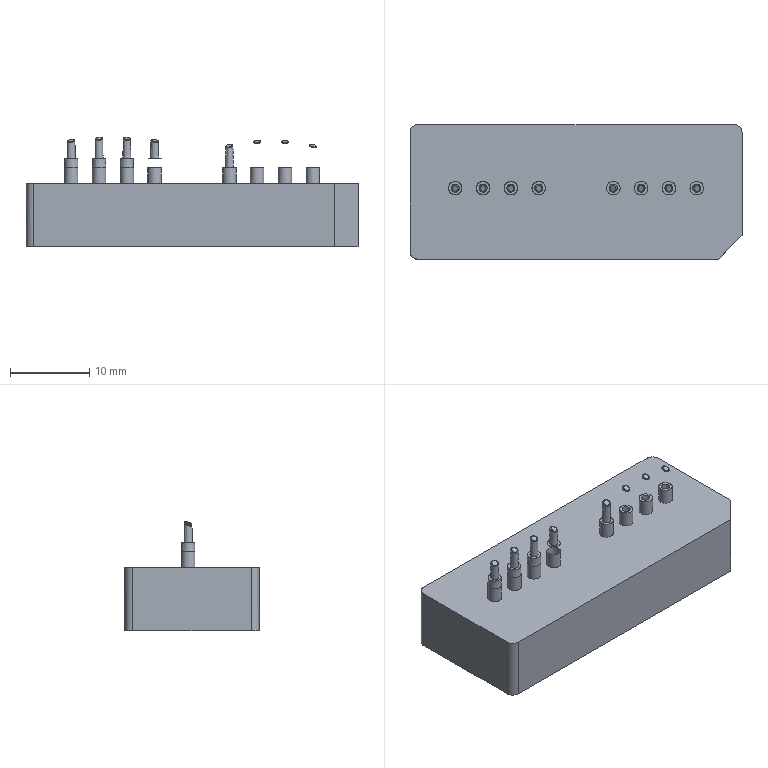NC program | PowerMill | posted by the shop | part box 42 x 17 x 13.856 mm
Lines 29045 to 29939 of 273708:
( TOOL ID   D10_1_1 )
( TOOL DIA. 10. TIP RAD 0 LENGTH 69. )
( Z = -6.06 )
T3 M6
T6
G91 G28 Z0
G0 G90 G54
M08
S8500 M3
X0 Y0 M8
G43 Z9.79 H3
X20.336 Y19.268
Z-4.86
G1 Z-6.06 F360
X20.127 Y13.997 F600
X6.597
X.484 Y5.107
X.565 Y5.157
X.642 Y5.215
X.852 Y5.391
X1.136 Y5.602
X1.42 Y5.789
X1.709 Y5.959
X1.987 Y6.103
X2.273 Y6.233
X2.555 Y6.346
X2.839 Y6.443
X3.128 Y6.526
X3.409 Y6.594
X3.691 Y6.647
X3.975 Y6.688
X4.259 Y6.716
X4.543 Y6.731
X4.826 Y6.732
X5.11 Y6.721
X5.394 Y6.697
X5.678 Y6.66
X5.962 Y6.61
X6.257 Y6.541
G3 X6.703 Y6.539 I.227 J.974
G1 X7.098 Y6.628
X7.382 Y6.674
X7.666 Y6.707
X7.95 Y6.726
X8.233 Y6.733
X8.517 Y6.727
X8.801 Y6.708
X9.085 Y6.676
X9.369 Y6.631
X9.598 Y6.584
X9.764 Y6.544
G3 X10.229 Y6.542 I.237 J.971
G1 X10.505 Y6.606
X10.789 Y6.658
X11.073 Y6.696
X11.356 Y6.72
X11.64 Y6.732
X11.924 Y6.731
X12.208 Y6.717
X12.492 Y6.69
X12.776 Y6.65
X13.06 Y6.596
X13.287 Y6.543
G3 X13.755 Y6.544 I.23 J.973
G1 X13.912 Y6.583
X14.196 Y6.639
X14.479 Y6.683
X14.763 Y6.712
X15.047 Y6.729
X15.331 Y6.733
X15.615 Y6.724
X15.899 Y6.702
X16.183 Y6.667
X16.467 Y6.619
X16.751 Y6.557
X17.095 Y6.463
X17.319 Y6.39
X17.601 Y6.286
X17.886 Y6.163
X18.086 Y6.067
X18.291 Y5.959
X18.454 Y5.866
X18.737 Y5.689
X19.022 Y5.488
X19.148 Y5.391
X19.355 Y5.221
X19.59 Y5.008
X19.796 Y4.802
X19.988 Y4.592
X20.158 Y4.39
X20.262 Y4.256
X20.466 Y3.971
X20.645 Y3.689
X20.726 Y3.55
X20.843 Y3.332
X20.946 Y3.121
X21.071 Y2.836
X21.177 Y2.554
G2 X21.347 Y1.986 I-5.759 J-2.034
G1 X21.411 Y1.703
X21.461 Y1.419
X21.497 Y1.135
X21.521 Y.851
X21.532 Y.568
X21.529 Y.284
X21.514 Y0
X21.486 Y-.284
X21.444 Y-.568
X21.389 Y-.851
X21.293 Y-1.234
X21.238 Y-1.419
X21.14 Y-1.703
X21.027 Y-1.986
X20.897 Y-2.27
X20.726 Y-2.595
X20.568 Y-2.858
X20.393 Y-3.121
X20.158 Y-3.435
X19.952 Y-3.679
X19.774 Y-3.871
X19.571 Y-4.071
X19.366 Y-4.256
X19.022 Y-4.533
X18.806 Y-4.688
X18.607 Y-4.818
X18.404 Y-4.939
X18.17 Y-5.069
X17.886 Y-5.208
X17.663 Y-5.305
X17.443 Y-5.391
X17.319 Y-5.436
X17.035 Y-5.526
X16.751 Y-5.602
X16.467 Y-5.664
X16.183 Y-5.712
X15.899 Y-5.747
X15.615 Y-5.769
X15.331 Y-5.778
X15.047 Y-5.774
X14.763 Y-5.758
X14.479 Y-5.727
X14.196 Y-5.684
X13.912 Y-5.628
X13.759 Y-5.59
G3 X13.288 Y-5.587 I-.241 J-.971
G1 X13.06 Y-5.641
X12.776 Y-5.695
X12.492 Y-5.735
X12.208 Y-5.762
X11.924 Y-5.776
X11.64 Y-5.777
X11.362 Y-5.766
X11.073 Y-5.741
X10.789 Y-5.703
X10.505 Y-5.651
X10.221 Y-5.586
G3 X9.749 Y-5.592 I-.224 J-.975
G1 X9.653 Y-5.617
X9.369 Y-5.676
X9.085 Y-5.721
X8.801 Y-5.753
X8.517 Y-5.772
X8.233 Y-5.778
X7.95 Y-5.772
X7.666 Y-5.752
X7.382 Y-5.719
X7.098 Y-5.673
X6.814 Y-5.613
X6.736 Y-5.593
G3 X6.246 Y-5.59 I-.251 J-.968
G1 X5.962 Y-5.654
X5.678 Y-5.705
X5.394 Y-5.742
X5.11 Y-5.766
X4.826 Y-5.778
X4.543 Y-5.776
X4.259 Y-5.761
X3.975 Y-5.734
X3.691 Y-5.692
X3.407 Y-5.638
X3.123 Y-5.57
X2.84 Y-5.488
X2.555 Y-5.39
X2.271 Y-5.278
X1.987 Y-5.148
X1.703 Y-5.001
X1.42 Y-4.835
X1.127 Y-4.641
X.852 Y-4.436
X.636 Y-4.258
G3 X-.636 Y-4.258 I-.636 J-.771
G1 X-.852 Y-4.436
X-1.127 Y-4.641
X-1.42 Y-4.835
X-1.703 Y-5.001
X-1.987 Y-5.148
X-2.271 Y-5.278
X-2.555 Y-5.39
X-2.84 Y-5.488
X-3.123 Y-5.57
X-3.407 Y-5.638
X-3.691 Y-5.692
X-3.975 Y-5.733
X-4.259 Y-5.761
X-4.543 Y-5.776
X-4.826 Y-5.778
X-5.11 Y-5.766
X-5.394 Y-5.742
X-5.678 Y-5.705
X-5.962 Y-5.654
X-6.246 Y-5.59
G3 X-6.736 Y-5.593 I-.239 J-.971
G1 X-6.814 Y-5.613
X-7.098 Y-5.673
X-7.382 Y-5.719
X-7.666 Y-5.752
X-7.95 Y-5.771
X-8.233 Y-5.778
X-8.517 Y-5.772
X-8.801 Y-5.753
X-9.085 Y-5.721
X-9.369 Y-5.676
X-9.653 Y-5.617
X-9.749 Y-5.592
G3 X-10.221 Y-5.586 I-.248 J-.969
G1 X-10.505 Y-5.651
X-10.789 Y-5.703
X-11.073 Y-5.741
X-11.363 Y-5.766
X-11.64 Y-5.777
X-11.924 Y-5.776
X-12.208 Y-5.762
X-12.492 Y-5.735
X-12.776 Y-5.695
X-13.06 Y-5.641
X-13.288 Y-5.587
G3 X-13.759 Y-5.59 I-.231 J-.973
G1 X-13.912 Y-5.628
X-14.196 Y-5.684
X-14.479 Y-5.727
X-14.763 Y-5.758
X-15.047 Y-5.774
X-15.331 Y-5.778
X-15.615 Y-5.769
X-15.899 Y-5.747
X-16.183 Y-5.712
X-16.467 Y-5.664
X-16.751 Y-5.602
X-17.035 Y-5.526
X-17.319 Y-5.436
X-17.661 Y-5.306
X-17.886 Y-5.208
X-18.17 Y-5.069
X-18.454 Y-4.911
X-18.598 Y-4.824
X-18.81 Y-4.685
X-19.022 Y-4.533
X-19.176 Y-4.414
X-19.366 Y-4.256
X-19.59 Y-4.053
X-19.774 Y-3.871
X-19.952 Y-3.679
X-20.158 Y-3.435
X-20.393 Y-3.121
X-20.569 Y-2.858
X-20.749 Y-2.554
X-20.896 Y-2.27
X-21.027 Y-1.986
X-21.14 Y-1.703
X-21.266 Y-1.326
X-21.293 Y-1.234
X-21.389 Y-.851
X-21.444 Y-.568
X-21.485 Y-.284
X-21.514 Y0
X-21.529 Y.284
X-21.531 Y.568
X-21.521 Y.851
X-21.498 Y1.135
X-21.461 Y1.419
X-21.411 Y1.703
X-21.347 Y1.986
G2 X-21.177 Y2.554 I6.096 J-1.516
G1 X-21.07 Y2.838
X-20.946 Y3.121
X-20.841 Y3.336
X-20.726 Y3.55
X-20.645 Y3.689
X-20.465 Y3.973
X-20.262 Y4.256
X-20.158 Y4.39
X-20.008 Y4.57
X-19.776 Y4.824
X-19.59 Y5.008
X-19.359 Y5.217
X-19.148 Y5.391
X-19.022 Y5.488
X-18.728 Y5.695
X-18.454 Y5.866
X-18.291 Y5.959
X-17.886 Y6.163
X-17.588 Y6.29
X-17.319 Y6.39
X-17.095 Y6.463
X-16.872 Y6.526
X-16.467 Y6.619
X-16.183 Y6.667
X-15.899 Y6.702
X-15.615 Y6.724
X-15.331 Y6.733
X-15.047 Y6.729
X-14.763 Y6.712
X-14.479 Y6.682
X-14.196 Y6.639
X-13.912 Y6.583
X-13.75 Y6.544
G3 X-13.286 Y6.543 I.234 J.972
G1 X-13.06 Y6.596
X-12.776 Y6.65
X-12.492 Y6.69
X-12.208 Y6.717
X-11.924 Y6.731
X-11.64 Y6.732
X-11.356 Y6.72
X-11.073 Y6.696
X-10.789 Y6.658
X-10.505 Y6.606
X-10.227 Y6.541
G3 X-9.781 Y6.539 I.228 J.974
G1 X-9.369 Y6.631
X-9.085 Y6.676
X-8.801 Y6.708
X-8.517 Y6.727
X-8.233 Y6.733
X-7.95 Y6.726
X-7.666 Y6.707
X-7.382 Y6.674
X-7.098 Y6.628
X-6.703 Y6.539
G3 X-6.256 Y6.541 I.219 J.976
G1 X-5.962 Y6.61
X-5.678 Y6.66
X-5.394 Y6.697
X-5.11 Y6.721
X-4.826 Y6.732
X-4.543 Y6.731
X-4.259 Y6.716
X-3.975 Y6.688
X-3.691 Y6.647
X-3.409 Y6.594
X-3.123 Y6.525
X-2.839 Y6.443
X-2.555 Y6.345
X-2.285 Y6.239
X-1.987 Y6.103
X-1.709 Y5.959
X-1.42 Y5.789
X-1.155 Y5.615
X-.852 Y5.391
X-.64 Y5.214
G3 X.484 Y5.107 I.641 J.768
G0 Z9.79
X0 Y0
X25.987 Y-14.768
Z-12.76
G1 Z-13.96 F360
G3 X22.452 Y-11.232 I-1.768 J1.768 F600
G1 X21.614 Y-12.07
X21.613 Y-12.071
X21.395 Y-12.279
X21.394 Y-12.28
X21.392 Y-12.281
X21.267 Y-12.39
X21.266 Y-12.391
X21.265 Y-12.392
X21.074 Y-12.545
X21.072 Y-12.546
X21.07 Y-12.547
X20.842 Y-12.711
X20.84 Y-12.712
X20.839 Y-12.713
X20.752 Y-12.77
X20.75 Y-12.771
X20.748 Y-12.772
X20.432 Y-12.96
X20.43 Y-12.961
X20.429 Y-12.962
X20.293 Y-13.033
X20.292
X20.291 Y-13.034
X20.11 Y-13.121
X20.108 Y-13.122
X20.106 Y-13.123
X19.79 Y-13.254
X19.787 Y-13.255
X19.785 Y-13.256
X19.499 Y-13.354
X19.496 Y-13.355
X19.494
X19.148 Y-13.449
X19.145
X19.142 Y-13.45
X18.826 Y-13.512
X18.824 Y-13.513
X18.821
X18.505 Y-13.555
X18.502
X18.5
X18.184 Y-13.577
X18.181
X18.179
X17.863 Y-13.58
X17.862
X-20.075 Y-13.579
X-20.077
X-20.078
X-20.394 Y-13.567
X-20.397
X-20.399
X-20.715 Y-13.538
X-20.717 Y-13.537
X-20.719
X-21.035 Y-13.491
X-21.037
X-21.039 Y-13.49
X-21.356 Y-13.427
X-21.358 Y-13.426
X-21.36
X-21.636 Y-13.356
X-21.638 Y-13.355
X-21.64 Y-13.354
X-21.996 Y-13.243
X-21.998 Y-13.242
X-22.001 Y-13.241
X-22.317 Y-13.121
X-22.319 Y-13.12
X-22.321
X-22.637 Y-12.978
X-22.639 Y-12.977
X-22.641 Y-12.976
X-22.957 Y-12.812
X-22.959 Y-12.811
X-22.961 Y-12.81
X-23.125 Y-12.715
X-23.127 Y-12.714
X-23.128
X-23.279 Y-12.62
X-23.28 Y-12.619
X-23.282 Y-12.618
X-23.598 Y-12.401
X-23.6 Y-12.399
X-23.602 Y-12.398
X-23.919 Y-12.149
X-23.92 Y-12.148
X-23.921 Y-12.147
X-24.005 Y-12.074
X-24.006 Y-12.073
X-24.008 Y-12.072
X-24.239 Y-11.858
X-24.241 Y-11.857
X-24.242 Y-11.856
X-24.344 Y-11.754
X-24.345 Y-11.753
X-24.346 Y-11.752
X-24.56 Y-11.522
X-24.561 Y-11.52
X-24.562 Y-11.519
X-24.636 Y-11.433
X-24.637 Y-11.432
Y-11.431
X-24.88 Y-11.126
X-24.882 Y-11.124
X-24.883 Y-11.122
X-25.11 Y-10.794
X-25.111 Y-10.793
X-25.112 Y-10.791
X-25.201 Y-10.648
X-25.202 Y-10.647
X-25.203 Y-10.646
X-25.303 Y-10.473
X-25.304 Y-10.471
X-25.305 Y-10.47
X-25.47 Y-10.154
X-25.471 Y-10.152
X-25.472 Y-10.149
X-25.614 Y-9.833
X-25.615 Y-9.831
X-25.616 Y-9.829
X-25.737 Y-9.513
X-25.738 Y-9.511
X-25.739 Y-9.509
X-25.84 Y-9.193
Y-9.19
X-25.841 Y-9.188
X-25.923 Y-8.872
X-25.924 Y-8.87
Y-8.868
X-25.988 Y-8.552
Y-8.55
Y-8.548
X-26.036 Y-8.232
Y-8.229
Y-8.227
X-26.065 Y-7.911
Y-7.909
X-26.066 Y-7.907
X-26.079 Y-7.591
Y-7.589
Y-7.587
Y7.587
Y7.589
Y7.591
X-26.066 Y7.907
Y7.909
Y7.911
X-26.036 Y8.227
Y8.229
Y8.231
X-25.989 Y8.548
Y8.55
X-25.988 Y8.552
X-25.924 Y8.868
Y8.87
X-25.923 Y8.872
X-25.843 Y9.179
Y9.182
X-25.842 Y9.184
X-25.738 Y9.509
Y9.511
X-25.737 Y9.513
X-25.616 Y9.829
X-25.615 Y9.831
X-25.614 Y9.833
X-25.472 Y10.149
X-25.471 Y10.152
X-25.47 Y10.154
X-25.305 Y10.47
X-25.304 Y10.471
X-25.303 Y10.473
X-25.203 Y10.646
X-25.202 Y10.647
X-25.201 Y10.648
X-25.112 Y10.791
X-25.111 Y10.793
X-25.11 Y10.794
X-24.892 Y11.111
X-24.89 Y11.113
X-24.889 Y11.115
X-24.638 Y11.431
X-24.637 Y11.432
X-24.636 Y11.434
X-24.562 Y11.519
X-24.561 Y11.521
X-24.56 Y11.522
X-24.346 Y11.752
X-24.345 Y11.753
X-24.344 Y11.754
X-24.242 Y11.856
X-24.241 Y11.857
X-24.239 Y11.858
X-24.007 Y12.072
X-24.006 Y12.073
X-24.005 Y12.074
X-23.921 Y12.146
X-23.92 Y12.147
X-23.919 Y12.148
X-23.61 Y12.392
X-23.608 Y12.394
X-23.605 Y12.396
X-23.282 Y12.618
X-23.28 Y12.619
X-23.279 Y12.62
X-23.128 Y12.714
X-23.127
X-23.125 Y12.715
X-22.961 Y12.81
X-22.959 Y12.811
X-22.957 Y12.812
X-22.641 Y12.976
X-22.639 Y12.977
X-22.637 Y12.978
X-22.321 Y13.12
X-22.319
X-22.317 Y13.121
X-22.001 Y13.241
X-21.998 Y13.242
X-21.996 Y13.243
X-21.68 Y13.343
X-21.678 Y13.344
X-21.676
X-21.36 Y13.426
X-21.358
X-21.355 Y13.427
X-21.039 Y13.49
X-21.037
X-21.035
X-20.719 Y13.537
X-20.717
X-20.715 Y13.538
X-20.399 Y13.566
X-20.397
X-20.395
X-20.079 Y13.579
X-20.077
X-20.075
X-.316
X20.075
X20.077
X20.078
X20.394 Y13.567
X20.397
X20.399
X20.715 Y13.538
X20.717 Y13.537
X20.719
X21.035 Y13.491
X21.037
X21.039 Y13.49
X21.356 Y13.427
X21.358 Y13.426
X21.36
X21.636 Y13.356
X21.638 Y13.355
X21.64 Y13.354
X21.996 Y13.243
X21.998 Y13.242
X22.001 Y13.241
X22.317 Y13.121
X22.319 Y13.12
X22.321
X22.637 Y12.978
X22.639 Y12.977
X22.641 Y12.976
X22.957 Y12.812
X22.959 Y12.811
X22.961 Y12.81
X23.125 Y12.715
X23.127 Y12.714
X23.128
X23.279 Y12.62
X23.28 Y12.619
X23.282 Y12.618
X23.598 Y12.401
X23.6 Y12.399
X23.602 Y12.398
X23.919 Y12.149
X23.92 Y12.148
X23.921 Y12.147
X24.005 Y12.074
X24.006 Y12.073
X24.008 Y12.072
X24.239 Y11.858
X24.241 Y11.857
X24.242 Y11.856
X24.344 Y11.754
X24.345 Y11.753
X24.346 Y11.752
X24.56 Y11.522
X24.561 Y11.52
X24.562 Y11.519
X24.636 Y11.433
X24.637 Y11.432
Y11.431
X24.88 Y11.126
X24.882 Y11.124
X24.883 Y11.122
X25.11 Y10.794
X25.111 Y10.793
X25.112 Y10.791
X25.201 Y10.648
X25.202 Y10.647
X25.203 Y10.646
X25.303 Y10.473
X25.304 Y10.471
X25.305 Y10.47
X25.47 Y10.154
X25.471 Y10.152
X25.472 Y10.149
X25.614 Y9.833
X25.615 Y9.831
X25.616 Y9.829
X25.737 Y9.513
X25.738 Y9.511
X25.739 Y9.509
X25.84 Y9.193
Y9.19
X25.841 Y9.188
X25.923 Y8.872
X25.924 Y8.87
Y8.868
X25.988 Y8.552
Y8.55
Y8.548
X26.036 Y8.232
Y8.229
Y8.227
X26.065 Y7.911
Y7.909
X26.066 Y7.907
X26.079 Y7.591
Y7.589
Y7.588
X26.08 Y-5.374
Y-5.375
X26.076 Y-5.692
Y-5.694
Y-5.696
X26.054 Y-6.012
Y-6.015
Y-6.017
X26.011 Y-6.334
Y-6.336
X26.01 Y-6.339
X25.947 Y-6.655
X25.946 Y-6.657
Y-6.66
X25.861 Y-6.976
X25.86 Y-6.979
X25.859 Y-6.981
X25.751 Y-7.297
Y-7.3
X25.75 Y-7.302
X25.617 Y-7.618
X25.616 Y-7.62
X25.615 Y-7.622
X25.522 Y-7.815
X25.521 Y-7.817
X25.52 Y-7.818
X25.455 Y-7.941
X25.454 Y-7.943
X25.453 Y-7.945
X25.264 Y-8.261
X25.263 Y-8.262
X25.262 Y-8.264
X25.2 Y-8.357
X25.199 Y-8.359
X25.198 Y-8.36
X25.038 Y-8.583
X25.036 Y-8.584
X25.035 Y-8.586
X24.88 Y-8.779
X24.879 Y-8.781
X24.878 Y-8.782
X24.77 Y-8.905
X24.769 Y-8.906
X24.768 Y-8.907
X24.559 Y-9.125
X24.558 Y-9.126
X22.452 Y-11.232
G3 X25.987 Y-14.768 I1.768 J-1.768
G1 X25.936 Y-14.706
G3 X22.4 Y-11.171 I-1.768 J1.768
G1 X21.558 Y-12.014
X21.34 Y-12.221
X21.215 Y-12.33
X21.024 Y-12.482
X20.795 Y-12.646
X20.708 Y-12.703
X20.391 Y-12.891
X20.256 Y-12.962
X20.075 Y-13.049
X19.759 Y-13.18
X19.473 Y-13.278
X19.127 Y-13.371
X18.811 Y-13.434
X18.495 Y-13.475
X18.178 Y-13.497
X17.862 Y-13.5
X-19.443
X-20.075 Y-13.499
X-20.391 Y-13.487
X-20.708 Y-13.458
X-21.024 Y-13.412
X-21.34 Y-13.348
X-21.616 Y-13.278
X-21.972 Y-13.167
X-22.288 Y-13.047
X-22.604 Y-12.905
X-22.921 Y-12.741
X-23.085 Y-12.646
X-23.237 Y-12.552
X-23.553 Y-12.335
X-23.869 Y-12.086
X-23.953 Y-12.014
X-24.185 Y-11.799
X-24.287 Y-11.697
X-24.501 Y-11.467
X-24.575 Y-11.381
X-24.817 Y-11.077
X-25.044 Y-10.749
X-25.134 Y-10.606
X-25.234 Y-10.433
X-25.399 Y-10.117
X-25.541 Y-9.801
X-25.662 Y-9.484
X-25.763 Y-9.168
X-25.846 Y-8.852
X-25.909 Y-8.536
X-25.957 Y-8.22
X-25.986 Y-7.904
X-25.999 Y-7.587
X-26. Y-7.271
Y7.271
X-25.999 Y7.587
X-25.986 Y7.904
X-25.957 Y8.22
X-25.91 Y8.536
X-25.846 Y8.852
X-25.766 Y9.159
X-25.662 Y9.484
X-25.541 Y9.801
X-25.399 Y10.117
X-25.234 Y10.433
X-25.134 Y10.606
X-25.044 Y10.749
X-24.826 Y11.065
X-24.576 Y11.381
X-24.501 Y11.467
X-24.287 Y11.697
X-24.185 Y11.799
X-23.953 Y12.014
X-23.869 Y12.085
X-23.56 Y12.33
X-23.237 Y12.552
X-23.085 Y12.646
X-22.921 Y12.741
X-22.604 Y12.905
X-22.288 Y13.047
X-21.972 Y13.167
X-21.656 Y13.267
X-21.34 Y13.348
X-21.024 Y13.411
X-20.708 Y13.458
X-20.391 Y13.486
X-20.075 Y13.499
X-19.759 Y13.5
X-.316
X19.127
X20.075 Y13.499
X20.391 Y13.487
X20.708 Y13.458
X21.024 Y13.412
X21.34 Y13.348
X21.616 Y13.278
X21.972 Y13.167
X22.288 Y13.047
X22.604 Y12.905
X22.921 Y12.741
X23.085 Y12.646
X23.237 Y12.552
X23.553 Y12.335
X23.869 Y12.086
X23.953 Y12.014
X24.185 Y11.799
X24.287 Y11.697
X24.501 Y11.467
X24.575 Y11.381
X24.817 Y11.077
X25.044 Y10.749
X25.134 Y10.606
X25.234 Y10.433
X25.399 Y10.117
X25.541 Y9.801
X25.662 Y9.484
X25.763 Y9.168
X25.846 Y8.852
X25.909 Y8.536
X25.957 Y8.22
X25.986 Y7.904
X25.999 Y7.587
X26. Y7.271
Y-5.374
X25.996 Y-5.691
X25.974 Y-6.007
X25.932 Y-6.323
X25.869 Y-6.639
X25.784 Y-6.955
X25.676 Y-7.271
X25.543 Y-7.587
X25.45 Y-7.78
X25.384 Y-7.904
X25.196 Y-8.22
X25.134 Y-8.313
X24.973 Y-8.536
X24.817 Y-8.729
X24.71 Y-8.852
X24.501 Y-9.07
X22.4 Y-11.171
G3 X25.936 Y-14.706 I1.768 J-1.768
G0 Z9.79
Z10.795
X0 Y0
M9
M5
M01